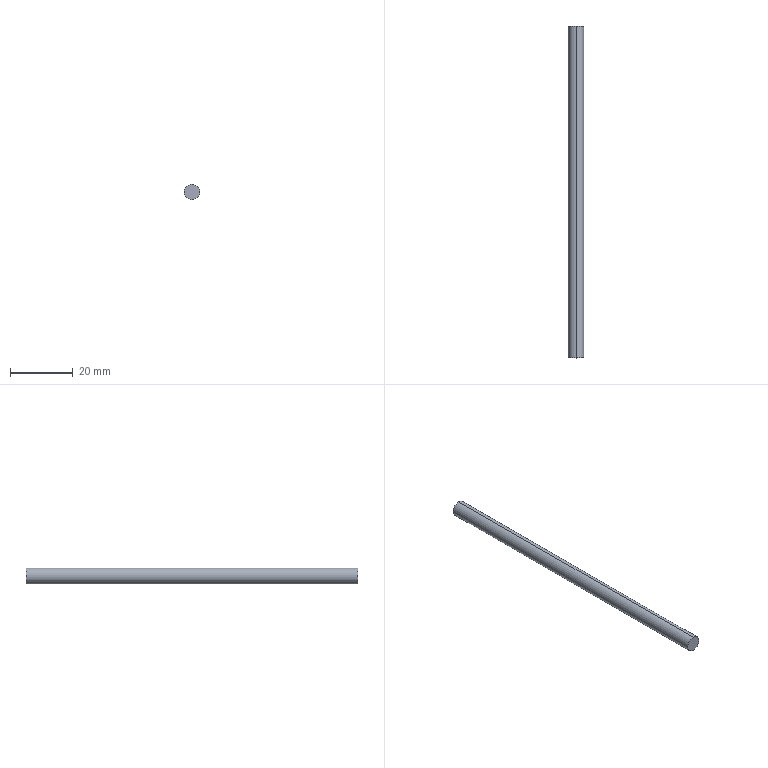Part | STEP file | Rear shaft short | 1 solid | 4 faces | box 5 x 106 x 5 mm | volume 2081 mm3 | cylinder 2 | plane 2 | commonest cylinder face diameters 5 x2
STEP:
#1=CARTESIAN_POINT('',(0.,0.,0.));
#2=DIRECTION('',(0.,0.,1.));
#3=DIRECTION('',(1.,0.,0.));
#4=AXIS2_PLACEMENT_3D('',#1,#2,#3);
#5=CARTESIAN_POINT('',(0.,106.,2.5));
#6=VERTEX_POINT('',#5);
#7=CARTESIAN_POINT('',(0.,106.,-2.5));
#8=VERTEX_POINT('',#7);
#9=CARTESIAN_POINT('',(0.,106.,0.));
#10=DIRECTION('',(0.,1.,0.));
#11=DIRECTION('',(0.,0.,1.));
#12=AXIS2_PLACEMENT_3D('',#9,#10,#11);
#13=CIRCLE('',#12,2.5);
#14=CARTESIAN_POINT('',(0.,106.,0.));
#15=DIRECTION('',(0.,-1.,0.));
#16=DIRECTION('',(0.,0.,-1.));
#17=AXIS2_PLACEMENT_3D('',#14,#15,#16);
#18=CYLINDRICAL_SURFACE('',#17,2.5);
#19=CARTESIAN_POINT('',(3.142,0.));
#20=DIRECTION('',(-1.,0.));
#21=VECTOR('',#20,1.);
#22=LINE('',#19,#21);
#23=(GEOMETRIC_REPRESENTATION_CONTEXT(2)PARAMETRIC_REPRESENTATION_CONTEXT()REPRESENTATION_CONTEXT('',''));
#24=DEFINITIONAL_REPRESENTATION('',(#22),#23);
#25=PCURVE('',#18,#24);
#26=CARTESIAN_POINT('',(0.,106.,0.));
#27=DIRECTION('',(0.,1.,0.));
#28=DIRECTION('',(0.,0.,1.));
#29=AXIS2_PLACEMENT_3D('',#26,#27,#28);
#30=PLANE('',#29);
#31=CARTESIAN_POINT('',(0.,0.));
#32=DIRECTION('',(1.,0.));
#33=AXIS2_PLACEMENT_2D('',#31,#32);
#34=CIRCLE('',#33,2.5);
#35=(GEOMETRIC_REPRESENTATION_CONTEXT(2)PARAMETRIC_REPRESENTATION_CONTEXT()REPRESENTATION_CONTEXT('',''));
#36=DEFINITIONAL_REPRESENTATION('',(#34),#35);
#37=PCURVE('',#30,#36);
#38=SURFACE_CURVE('',#13,(#25,#37),.PCURVE_S1.);
#39=EDGE_CURVE('',#6,#8,#38,.T.);
#40=ORIENTED_EDGE('',*,*,#39,.F.);
#41=CARTESIAN_POINT('',(0.,0.,2.5));
#42=VERTEX_POINT('',#41);
#43=CARTESIAN_POINT('',(0.,106.,2.5));
#44=DIRECTION('',(0.,-1.,0.));
#45=VECTOR('',#44,1.);
#46=LINE('',#43,#45);
#47=CARTESIAN_POINT('',(3.142,0.));
#48=DIRECTION('',(0.,1.));
#49=VECTOR('',#48,1.);
#50=LINE('',#47,#49);
#51=(GEOMETRIC_REPRESENTATION_CONTEXT(2)PARAMETRIC_REPRESENTATION_CONTEXT()REPRESENTATION_CONTEXT('',''));
#52=DEFINITIONAL_REPRESENTATION('',(#50),#51);
#53=PCURVE('',#18,#52);
#54=CARTESIAN_POINT('',(0.,106.,0.));
#55=DIRECTION('',(0.,-1.,0.));
#56=DIRECTION('',(0.,0.,-1.));
#57=AXIS2_PLACEMENT_3D('',#54,#55,#56);
#58=CYLINDRICAL_SURFACE('',#57,2.5);
#59=CARTESIAN_POINT('',(3.142,0.));
#60=DIRECTION('',(0.,1.));
#61=VECTOR('',#60,1.);
#62=LINE('',#59,#61);
#63=(GEOMETRIC_REPRESENTATION_CONTEXT(2)PARAMETRIC_REPRESENTATION_CONTEXT()REPRESENTATION_CONTEXT('',''));
#64=DEFINITIONAL_REPRESENTATION('',(#62),#63);
#65=PCURVE('',#58,#64);
#66=SURFACE_CURVE('',#46,(#53,#65),.PCURVE_S1.);
#67=EDGE_CURVE('',#6,#42,#66,.T.);
#68=ORIENTED_EDGE('',*,*,#67,.T.);
#69=CARTESIAN_POINT('',(0.,0.,-2.5));
#70=VERTEX_POINT('',#69);
#71=CARTESIAN_POINT('',(0.,0.,0.));
#72=DIRECTION('',(0.,1.,0.));
#73=DIRECTION('',(0.,0.,1.));
#74=AXIS2_PLACEMENT_3D('',#71,#72,#73);
#75=CIRCLE('',#74,2.5);
#76=CARTESIAN_POINT('',(3.142,106.));
#77=DIRECTION('',(-1.,0.));
#78=VECTOR('',#77,1.);
#79=LINE('',#76,#78);
#80=(GEOMETRIC_REPRESENTATION_CONTEXT(2)PARAMETRIC_REPRESENTATION_CONTEXT()REPRESENTATION_CONTEXT('',''));
#81=DEFINITIONAL_REPRESENTATION('',(#79),#80);
#82=PCURVE('',#18,#81);
#83=CARTESIAN_POINT('',(0.,0.,0.));
#84=DIRECTION('',(0.,1.,0.));
#85=DIRECTION('',(0.,0.,1.));
#86=AXIS2_PLACEMENT_3D('',#83,#84,#85);
#87=PLANE('',#86);
#88=CARTESIAN_POINT('',(0.,0.));
#89=DIRECTION('',(1.,0.));
#90=AXIS2_PLACEMENT_2D('',#88,#89);
#91=CIRCLE('',#90,2.5);
#92=(GEOMETRIC_REPRESENTATION_CONTEXT(2)PARAMETRIC_REPRESENTATION_CONTEXT()REPRESENTATION_CONTEXT('',''));
#93=DEFINITIONAL_REPRESENTATION('',(#91),#92);
#94=PCURVE('',#87,#93);
#95=SURFACE_CURVE('',#75,(#82,#94),.PCURVE_S1.);
#96=EDGE_CURVE('',#42,#70,#95,.T.);
#97=ORIENTED_EDGE('',*,*,#96,.T.);
#98=CARTESIAN_POINT('',(0.,106.,-2.5));
#99=DIRECTION('',(0.,-1.,0.));
#100=VECTOR('',#99,1.);
#101=LINE('',#98,#100);
#102=CARTESIAN_POINT('',(0.,0.));
#103=DIRECTION('',(0.,1.));
#104=VECTOR('',#103,1.);
#105=LINE('',#102,#104);
#106=(GEOMETRIC_REPRESENTATION_CONTEXT(2)PARAMETRIC_REPRESENTATION_CONTEXT()REPRESENTATION_CONTEXT('',''));
#107=DEFINITIONAL_REPRESENTATION('',(#105),#106);
#108=PCURVE('',#18,#107);
#109=CARTESIAN_POINT('',(6.283,0.));
#110=DIRECTION('',(0.,1.));
#111=VECTOR('',#110,1.);
#112=LINE('',#109,#111);
#113=(GEOMETRIC_REPRESENTATION_CONTEXT(2)PARAMETRIC_REPRESENTATION_CONTEXT()REPRESENTATION_CONTEXT('',''));
#114=DEFINITIONAL_REPRESENTATION('',(#112),#113);
#115=PCURVE('',#58,#114);
#116=SURFACE_CURVE('',#101,(#108,#115),.PCURVE_S1.);
#117=EDGE_CURVE('',#8,#70,#116,.T.);
#118=ORIENTED_EDGE('',*,*,#117,.F.);
#119=EDGE_LOOP('',(#40,#68,#97,#118));
#120=FACE_BOUND('',#119,.T.);
#121=ADVANCED_FACE('',(#120),#18,.T.);
#122=ORIENTED_EDGE('',*,*,#67,.F.);
#123=CARTESIAN_POINT('',(0.,106.,0.));
#124=DIRECTION('',(0.,1.,0.));
#125=DIRECTION('',(0.,0.,1.));
#126=AXIS2_PLACEMENT_3D('',#123,#124,#125);
#127=CIRCLE('',#126,2.5);
#128=CARTESIAN_POINT('',(9.425,0.));
#129=DIRECTION('',(-1.,0.));
#130=VECTOR('',#129,1.);
#131=LINE('',#128,#130);
#132=(GEOMETRIC_REPRESENTATION_CONTEXT(2)PARAMETRIC_REPRESENTATION_CONTEXT()REPRESENTATION_CONTEXT('',''));
#133=DEFINITIONAL_REPRESENTATION('',(#131),#132);
#134=PCURVE('',#58,#133);
#135=CARTESIAN_POINT('',(0.,0.));
#136=DIRECTION('',(1.,0.));
#137=AXIS2_PLACEMENT_2D('',#135,#136);
#138=CIRCLE('',#137,2.5);
#139=(GEOMETRIC_REPRESENTATION_CONTEXT(2)PARAMETRIC_REPRESENTATION_CONTEXT()REPRESENTATION_CONTEXT('',''));
#140=DEFINITIONAL_REPRESENTATION('',(#138),#139);
#141=PCURVE('',#30,#140);
#142=SURFACE_CURVE('',#127,(#134,#141),.PCURVE_S1.);
#143=EDGE_CURVE('',#8,#6,#142,.T.);
#144=ORIENTED_EDGE('',*,*,#143,.F.);
#145=ORIENTED_EDGE('',*,*,#117,.T.);
#146=CARTESIAN_POINT('',(0.,0.,0.));
#147=DIRECTION('',(0.,1.,0.));
#148=DIRECTION('',(0.,0.,1.));
#149=AXIS2_PLACEMENT_3D('',#146,#147,#148);
#150=CIRCLE('',#149,2.5);
#151=CARTESIAN_POINT('',(9.425,106.));
#152=DIRECTION('',(-1.,0.));
#153=VECTOR('',#152,1.);
#154=LINE('',#151,#153);
#155=(GEOMETRIC_REPRESENTATION_CONTEXT(2)PARAMETRIC_REPRESENTATION_CONTEXT()REPRESENTATION_CONTEXT('',''));
#156=DEFINITIONAL_REPRESENTATION('',(#154),#155);
#157=PCURVE('',#58,#156);
#158=CARTESIAN_POINT('',(0.,0.));
#159=DIRECTION('',(1.,0.));
#160=AXIS2_PLACEMENT_2D('',#158,#159);
#161=CIRCLE('',#160,2.5);
#162=(GEOMETRIC_REPRESENTATION_CONTEXT(2)PARAMETRIC_REPRESENTATION_CONTEXT()REPRESENTATION_CONTEXT('',''));
#163=DEFINITIONAL_REPRESENTATION('',(#161),#162);
#164=PCURVE('',#87,#163);
#165=SURFACE_CURVE('',#150,(#157,#164),.PCURVE_S1.);
#166=EDGE_CURVE('',#70,#42,#165,.T.);
#167=ORIENTED_EDGE('',*,*,#166,.T.);
#168=EDGE_LOOP('',(#122,#144,#145,#167));
#169=FACE_BOUND('',#168,.T.);
#170=ADVANCED_FACE('',(#169),#58,.T.);
#171=ORIENTED_EDGE('',*,*,#143,.T.);
#172=ORIENTED_EDGE('',*,*,#39,.T.);
#173=EDGE_LOOP('',(#171,#172));
#174=FACE_BOUND('',#173,.T.);
#175=ADVANCED_FACE('',(#174),#30,.T.);
#176=ORIENTED_EDGE('',*,*,#166,.F.);
#177=ORIENTED_EDGE('',*,*,#96,.F.);
#178=EDGE_LOOP('',(#176,#177));
#179=FACE_BOUND('',#178,.T.);
#180=ADVANCED_FACE('',(#179),#87,.F.);
#181=CLOSED_SHELL('',(#121,#170,#175,#180));
#182=MANIFOLD_SOLID_BREP('',#181);
#183=(LENGTH_UNIT()NAMED_UNIT(*)SI_UNIT(.MILLI.,.METRE.));
#184=UNCERTAINTY_MEASURE_WITH_UNIT(LENGTH_MEASURE(0.0000001),#183,'','');
#185=(NAMED_UNIT(*)PLANE_ANGLE_UNIT()SI_UNIT($,.RADIAN.));
#186=(NAMED_UNIT(*)SI_UNIT($,.STERADIAN.)SOLID_ANGLE_UNIT());
#187=(GEOMETRIC_REPRESENTATION_CONTEXT(3)GLOBAL_UNCERTAINTY_ASSIGNED_CONTEXT((#184))GLOBAL_UNIT_ASSIGNED_CONTEXT((#183,#185,#186))REPRESENTATION_CONTEXT('',''));
#188=ADVANCED_BREP_SHAPE_REPRESENTATION('',(#4,#182),#187);